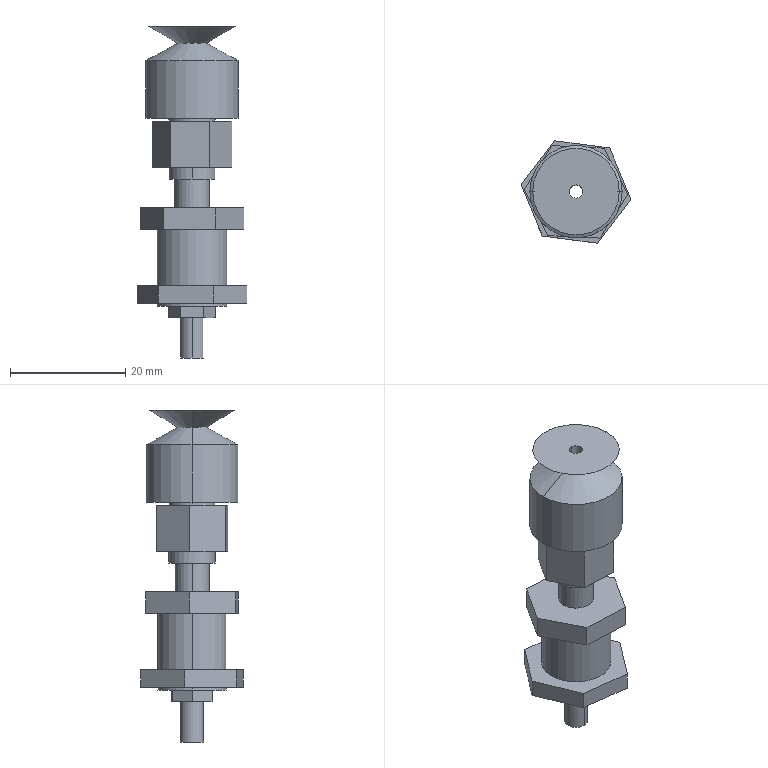Part | STEP file | Suction nozzle SRKN10+SRP15 | 2 solids | 59 faces | box 19.039 x 17.729 x 57.5 mm | volume 6399 mm3 | plane 37 | cylinder 16 | cone 6 | commonest cylinder face diameters 8 x4 12 x4 2.3 x2 4 x2 6 x2 16 x2